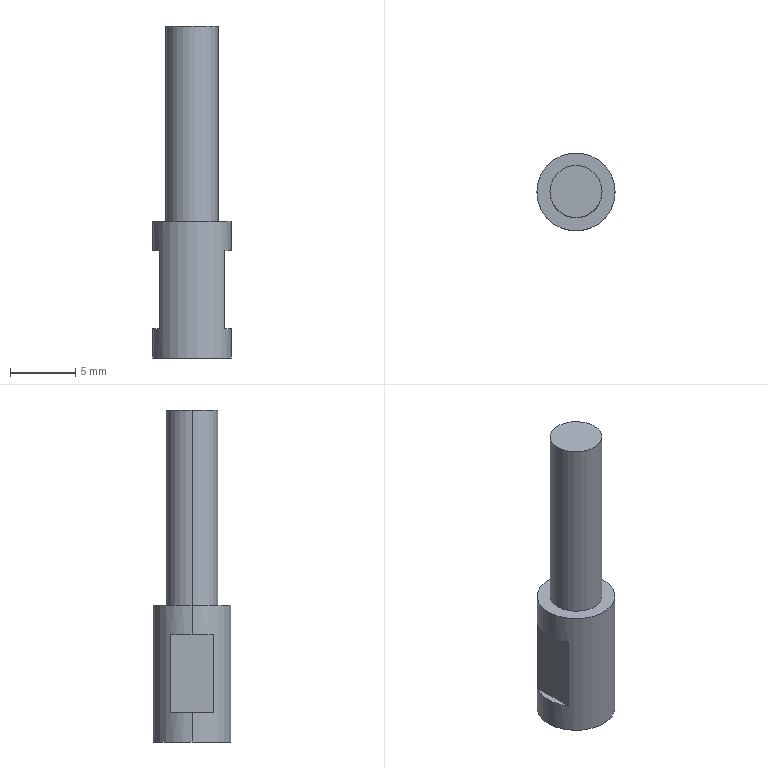Part | STEP file | GLSJ-10-20 | 1 solid | 17 faces | box 6 x 6 x 25.5 mm | volume 383.515 mm3 | plane 9 | cylinder 6 | cone 2 | commonest cylinder face diameters 3.3 x2 4 x2 6 x2
STEP:
#1=CARTESIAN_POINT('',(0.,0.,0.));
#2=DIRECTION('',(0.,0.,1.));
#3=DIRECTION('',(1.,0.,0.));
#4=AXIS2_PLACEMENT_3D('',#1,#2,#3);
#5=CARTESIAN_POINT('',(-1.65,0.,10.));
#6=VERTEX_POINT('',#5);
#7=CARTESIAN_POINT('',(-1.65,0.,0.));
#8=VERTEX_POINT('',#7);
#9=CARTESIAN_POINT('',(-1.65,0.,0.));
#10=DIRECTION('',(0.,0.,-1.));
#11=VECTOR('',#10,1.);
#12=LINE('',#9,#11);
#13=CARTESIAN_POINT('',(0.,0.,0.));
#14=DIRECTION('',(0.,0.,-1.));
#15=DIRECTION('',(-1.,0.,0.));
#16=AXIS2_PLACEMENT_3D('',#13,#14,#15);
#17=CYLINDRICAL_SURFACE('',#16,1.65);
#18=CARTESIAN_POINT('',(6.283,0.));
#19=DIRECTION('',(0.,1.));
#20=VECTOR('',#19,1.);
#21=LINE('',#18,#20);
#22=(GEOMETRIC_REPRESENTATION_CONTEXT(2)PARAMETRIC_REPRESENTATION_CONTEXT()REPRESENTATION_CONTEXT('',''));
#23=DEFINITIONAL_REPRESENTATION('',(#21),#22);
#24=PCURVE('',#17,#23);
#25=CARTESIAN_POINT('',(0.,0.,0.));
#26=DIRECTION('',(0.,0.,-1.));
#27=DIRECTION('',(-1.,0.,0.));
#28=AXIS2_PLACEMENT_3D('',#25,#26,#27);
#29=CYLINDRICAL_SURFACE('',#28,1.65);
#30=CARTESIAN_POINT('',(0.,0.));
#31=DIRECTION('',(0.,1.));
#32=VECTOR('',#31,1.);
#33=LINE('',#30,#32);
#34=(GEOMETRIC_REPRESENTATION_CONTEXT(2)PARAMETRIC_REPRESENTATION_CONTEXT()REPRESENTATION_CONTEXT('',''));
#35=DEFINITIONAL_REPRESENTATION('',(#33),#34);
#36=PCURVE('',#29,#35);
#37=SURFACE_CURVE('',#12,(#24,#36),.PCURVE_S1.);
#38=EDGE_CURVE('',#6,#8,#37,.T.);
#39=ORIENTED_EDGE('',*,*,#38,.T.);
#40=CARTESIAN_POINT('',(1.65,0.,0.));
#41=VERTEX_POINT('',#40);
#42=CARTESIAN_POINT('',(0.,0.,0.));
#43=DIRECTION('',(0.,0.,-1.));
#44=DIRECTION('',(-1.,0.,0.));
#45=AXIS2_PLACEMENT_3D('',#42,#43,#44);
#46=CIRCLE('',#45,1.65);
#47=CARTESIAN_POINT('',(0.,0.));
#48=DIRECTION('',(1.,0.));
#49=VECTOR('',#48,1.);
#50=LINE('',#47,#49);
#51=(GEOMETRIC_REPRESENTATION_CONTEXT(2)PARAMETRIC_REPRESENTATION_CONTEXT()REPRESENTATION_CONTEXT('',''));
#52=DEFINITIONAL_REPRESENTATION('',(#50),#51);
#53=PCURVE('',#17,#52);
#54=CARTESIAN_POINT('',(0.,0.,0.));
#55=DIRECTION('',(0.,0.,1.));
#56=DIRECTION('',(1.,0.,0.));
#57=AXIS2_PLACEMENT_3D('',#54,#55,#56);
#58=PLANE('',#57);
#59=CARTESIAN_POINT('',(-1.65,0.));
#60=CARTESIAN_POINT('',(-1.65,2.858));
#61=CARTESIAN_POINT('',(0.825,1.429));
#62=CARTESIAN_POINT('',(3.3,0.));
#63=CARTESIAN_POINT('',(0.825,-1.429));
#64=CARTESIAN_POINT('',(-1.65,-2.858));
#65=CARTESIAN_POINT('',(-1.65,0.));
#66=(BOUNDED_CURVE()B_SPLINE_CURVE(2,(#59,#60,#61,#62,#63,#64,#65),.UNSPECIFIED.,.T.,.F.)B_SPLINE_CURVE_WITH_KNOTS((1,2,2,2,2,1),(-2.094,0.,2.094,4.189,6.283,8.378),.UNSPECIFIED.)CURVE()GEOMETRIC_REPRESENTATION_ITEM()RATIONAL_B_SPLINE_CURVE((1.,0.5,1.,0.5,1.,0.5,1.))REPRESENTATION_ITEM(''));
#67=(GEOMETRIC_REPRESENTATION_CONTEXT(2)PARAMETRIC_REPRESENTATION_CONTEXT()REPRESENTATION_CONTEXT('',''));
#68=DEFINITIONAL_REPRESENTATION('',(#66),#67);
#69=PCURVE('',#58,#68);
#70=SURFACE_CURVE('',#46,(#53,#69),.PCURVE_S1.);
#71=EDGE_CURVE('',#41,#8,#70,.T.);
#72=ORIENTED_EDGE('',*,*,#71,.F.);
#73=CARTESIAN_POINT('',(1.65,0.,10.));
#74=VERTEX_POINT('',#73);
#75=CARTESIAN_POINT('',(1.65,0.,0.));
#76=DIRECTION('',(0.,0.,-1.));
#77=VECTOR('',#76,1.);
#78=LINE('',#75,#77);
#79=CARTESIAN_POINT('',(3.142,0.));
#80=DIRECTION('',(0.,1.));
#81=VECTOR('',#80,1.);
#82=LINE('',#79,#81);
#83=(GEOMETRIC_REPRESENTATION_CONTEXT(2)PARAMETRIC_REPRESENTATION_CONTEXT()REPRESENTATION_CONTEXT('',''));
#84=DEFINITIONAL_REPRESENTATION('',(#82),#83);
#85=PCURVE('',#17,#84);
#86=CARTESIAN_POINT('',(3.142,0.));
#87=DIRECTION('',(0.,1.));
#88=VECTOR('',#87,1.);
#89=LINE('',#86,#88);
#90=(GEOMETRIC_REPRESENTATION_CONTEXT(2)PARAMETRIC_REPRESENTATION_CONTEXT()REPRESENTATION_CONTEXT('',''));
#91=DEFINITIONAL_REPRESENTATION('',(#89),#90);
#92=PCURVE('',#29,#91);
#93=SURFACE_CURVE('',#78,(#85,#92),.PCURVE_S1.);
#94=EDGE_CURVE('',#74,#41,#93,.T.);
#95=ORIENTED_EDGE('',*,*,#94,.F.);
#96=CARTESIAN_POINT('',(0.,0.,10.));
#97=DIRECTION('',(0.,0.,-1.));
#98=DIRECTION('',(-1.,0.,0.));
#99=AXIS2_PLACEMENT_3D('',#96,#97,#98);
#100=CIRCLE('',#99,1.65);
#101=CARTESIAN_POINT('',(0.,-10.));
#102=DIRECTION('',(1.,0.));
#103=VECTOR('',#102,1.);
#104=LINE('',#101,#103);
#105=(GEOMETRIC_REPRESENTATION_CONTEXT(2)PARAMETRIC_REPRESENTATION_CONTEXT()REPRESENTATION_CONTEXT('',''));
#106=DEFINITIONAL_REPRESENTATION('',(#104),#105);
#107=PCURVE('',#17,#106);
#108=CARTESIAN_POINT('',(0.,0.,10.));
#109=DIRECTION('',(0.,0.,-1.));
#110=DIRECTION('',(-1.,0.,0.));
#111=AXIS2_PLACEMENT_3D('',#108,#109,#110);
#112=CONICAL_SURFACE('',#111,1.65,1.03);
#113=CARTESIAN_POINT('',(0.,0.));
#114=DIRECTION('',(1.,0.));
#115=VECTOR('',#114,1.);
#116=LINE('',#113,#115);
#117=(GEOMETRIC_REPRESENTATION_CONTEXT(2)PARAMETRIC_REPRESENTATION_CONTEXT()REPRESENTATION_CONTEXT('',''));
#118=DEFINITIONAL_REPRESENTATION('',(#116),#117);
#119=PCURVE('',#112,#118);
#120=SURFACE_CURVE('',#100,(#107,#119),.PCURVE_S1.);
#121=EDGE_CURVE('',#74,#6,#120,.T.);
#122=ORIENTED_EDGE('',*,*,#121,.T.);
#123=EDGE_LOOP('',(#39,#72,#95,#122));
#124=FACE_BOUND('',#123,.F.);
#125=ADVANCED_FACE('',(#124),#17,.F.);
#126=ORIENTED_EDGE('',*,*,#121,.F.);
#127=CARTESIAN_POINT('',(0.,0.,10.991));
#128=VERTEX_POINT('',#127);
#129=CARTESIAN_POINT('',(1.65,0.,10.));
#130=DIRECTION('',(0.8572,0.,-0.515));
#131=VECTOR('',#130,1.);
#132=LINE('',#129,#131);
#133=CARTESIAN_POINT('',(3.142,-0.9914));
#134=CARTESIAN_POINT('',(3.142,-0.9764));
#135=CARTESIAN_POINT('',(3.142,-0.9464));
#136=CARTESIAN_POINT('',(3.142,-0.9013));
#137=CARTESIAN_POINT('',(3.142,-0.8562));
#138=CARTESIAN_POINT('',(3.142,-0.8112));
#139=CARTESIAN_POINT('',(3.142,-0.7661));
#140=CARTESIAN_POINT('',(3.142,-0.721));
#141=CARTESIAN_POINT('',(3.142,-0.676));
#142=CARTESIAN_POINT('',(3.142,-0.6309));
#143=CARTESIAN_POINT('',(3.142,-0.5858));
#144=CARTESIAN_POINT('',(3.142,-0.5408));
#145=CARTESIAN_POINT('',(3.142,-0.4957));
#146=CARTESIAN_POINT('',(3.142,-0.4506));
#147=CARTESIAN_POINT('',(3.142,-0.4056));
#148=CARTESIAN_POINT('',(3.142,-0.3605));
#149=CARTESIAN_POINT('',(3.142,-0.3155));
#150=CARTESIAN_POINT('',(3.142,-0.2704));
#151=CARTESIAN_POINT('',(3.142,-0.2253));
#152=CARTESIAN_POINT('',(3.142,-0.1803));
#153=CARTESIAN_POINT('',(3.142,-0.1352));
#154=CARTESIAN_POINT('',(3.142,-0.09013));
#155=CARTESIAN_POINT('',(3.142,-0.04506));
#156=CARTESIAN_POINT('',(3.142,-0.01502));
#157=CARTESIAN_POINT('',(3.142,0.));
#158=B_SPLINE_CURVE_WITH_KNOTS('',3,(#133,#134,#135,#136,#137,#138,#139,#140,#141,#142,#143,#144,#145,#146,#147,#148,#149,#150,#151,#152,#153,#154,#155,#156,#157),.UNSPECIFIED.,.F.,.F.,(4,1,1,1,1,1,1,1,1,1,1,1,1,1,1,1,1,1,1,1,1,1,4),(-1.925,-1.837,-1.75,-1.662,-1.575,-1.487,-1.4,-1.312,-1.225,-1.137,-1.05,-0.9625,-0.875,-0.7875,-0.7,-0.6125,-0.525,-0.4375,-0.35,-0.2625,-0.175,-0.0875,0.),.QUASI_UNIFORM_KNOTS.);
#159=(GEOMETRIC_REPRESENTATION_CONTEXT(2)PARAMETRIC_REPRESENTATION_CONTEXT()REPRESENTATION_CONTEXT('',''));
#160=DEFINITIONAL_REPRESENTATION('',(#158),#159);
#161=PCURVE('',#112,#160);
#162=CARTESIAN_POINT('',(0.,0.,10.));
#163=DIRECTION('',(0.,0.,-1.));
#164=DIRECTION('',(-1.,0.,0.));
#165=AXIS2_PLACEMENT_3D('',#162,#163,#164);
#166=CONICAL_SURFACE('',#165,1.65,1.03);
#167=CARTESIAN_POINT('',(3.142,-0.9914));
#168=CARTESIAN_POINT('',(3.142,-0.9764));
#169=CARTESIAN_POINT('',(3.142,-0.9464));
#170=CARTESIAN_POINT('',(3.142,-0.9013));
#171=CARTESIAN_POINT('',(3.142,-0.8562));
#172=CARTESIAN_POINT('',(3.142,-0.8112));
#173=CARTESIAN_POINT('',(3.142,-0.7661));
#174=CARTESIAN_POINT('',(3.142,-0.721));
#175=CARTESIAN_POINT('',(3.142,-0.676));
#176=CARTESIAN_POINT('',(3.142,-0.6309));
#177=CARTESIAN_POINT('',(3.142,-0.5858));
#178=CARTESIAN_POINT('',(3.142,-0.5408));
#179=CARTESIAN_POINT('',(3.142,-0.4957));
#180=CARTESIAN_POINT('',(3.142,-0.4506));
#181=CARTESIAN_POINT('',(3.142,-0.4056));
#182=CARTESIAN_POINT('',(3.142,-0.3605));
#183=CARTESIAN_POINT('',(3.142,-0.3155));
#184=CARTESIAN_POINT('',(3.142,-0.2704));
#185=CARTESIAN_POINT('',(3.142,-0.2253));
#186=CARTESIAN_POINT('',(3.142,-0.1803));
#187=CARTESIAN_POINT('',(3.142,-0.1352));
#188=CARTESIAN_POINT('',(3.142,-0.09013));
#189=CARTESIAN_POINT('',(3.142,-0.04506));
#190=CARTESIAN_POINT('',(3.142,-0.01502));
#191=CARTESIAN_POINT('',(3.142,0.));
#192=B_SPLINE_CURVE_WITH_KNOTS('',3,(#167,#168,#169,#170,#171,#172,#173,#174,#175,#176,#177,#178,#179,#180,#181,#182,#183,#184,#185,#186,#187,#188,#189,#190,#191),.UNSPECIFIED.,.F.,.F.,(4,1,1,1,1,1,1,1,1,1,1,1,1,1,1,1,1,1,1,1,1,1,4),(-1.925,-1.837,-1.75,-1.662,-1.575,-1.487,-1.4,-1.312,-1.225,-1.137,-1.05,-0.9625,-0.875,-0.7875,-0.7,-0.6125,-0.525,-0.4375,-0.35,-0.2625,-0.175,-0.0875,0.),.QUASI_UNIFORM_KNOTS.);
#193=(GEOMETRIC_REPRESENTATION_CONTEXT(2)PARAMETRIC_REPRESENTATION_CONTEXT()REPRESENTATION_CONTEXT('',''));
#194=DEFINITIONAL_REPRESENTATION('',(#192),#193);
#195=PCURVE('',#166,#194);
#196=SURFACE_CURVE('',#132,(#161,#195),.PCURVE_S1.);
#197=EDGE_CURVE('',#128,#74,#196,.T.);
#198=ORIENTED_EDGE('',*,*,#197,.F.);
#199=CARTESIAN_POINT('',(-1.65,0.,10.));
#200=DIRECTION('',(-0.8572,0.,-0.515));
#201=VECTOR('',#200,1.);
#202=LINE('',#199,#201);
#203=CARTESIAN_POINT('',(6.283,0.));
#204=DIRECTION('',(0.,1.));
#205=VECTOR('',#204,1.);
#206=LINE('',#203,#205);
#207=(GEOMETRIC_REPRESENTATION_CONTEXT(2)PARAMETRIC_REPRESENTATION_CONTEXT()REPRESENTATION_CONTEXT('',''));
#208=DEFINITIONAL_REPRESENTATION('',(#206),#207);
#209=PCURVE('',#112,#208);
#210=CARTESIAN_POINT('',(0.,0.));
#211=DIRECTION('',(0.,1.));
#212=VECTOR('',#211,1.);
#213=LINE('',#210,#212);
#214=(GEOMETRIC_REPRESENTATION_CONTEXT(2)PARAMETRIC_REPRESENTATION_CONTEXT()REPRESENTATION_CONTEXT('',''));
#215=DEFINITIONAL_REPRESENTATION('',(#213),#214);
#216=PCURVE('',#166,#215);
#217=SURFACE_CURVE('',#202,(#209,#216),.PCURVE_S1.);
#218=EDGE_CURVE('',#128,#6,#217,.T.);
#219=ORIENTED_EDGE('',*,*,#218,.T.);
#220=EDGE_LOOP('',(#126,#198,#219));
#221=FACE_BOUND('',#220,.F.);
#222=ADVANCED_FACE('',(#221),#112,.F.);
#223=CARTESIAN_POINT('',(2.,0.,10.5));
#224=VERTEX_POINT('',#223);
#225=CARTESIAN_POINT('',(-2.,0.,10.5));
#226=VERTEX_POINT('',#225);
#227=CARTESIAN_POINT('',(0.,0.,10.5));
#228=DIRECTION('',(0.,0.,1.));
#229=DIRECTION('',(1.,0.,0.));
#230=AXIS2_PLACEMENT_3D('',#227,#228,#229);
#231=CIRCLE('',#230,2.);
#232=CARTESIAN_POINT('',(0.,0.,10.5));
#233=DIRECTION('',(0.,0.,1.));
#234=DIRECTION('',(1.,0.,0.));
#235=AXIS2_PLACEMENT_3D('',#232,#233,#234);
#236=CYLINDRICAL_SURFACE('',#235,2.);
#237=CARTESIAN_POINT('',(0.,0.));
#238=DIRECTION('',(1.,0.));
#239=VECTOR('',#238,1.);
#240=LINE('',#237,#239);
#241=(GEOMETRIC_REPRESENTATION_CONTEXT(2)PARAMETRIC_REPRESENTATION_CONTEXT()REPRESENTATION_CONTEXT('',''));
#242=DEFINITIONAL_REPRESENTATION('',(#240),#241);
#243=PCURVE('',#236,#242);
#244=CARTESIAN_POINT('',(0.,0.,10.5));
#245=DIRECTION('',(0.,0.,1.));
#246=DIRECTION('',(1.,0.,0.));
#247=AXIS2_PLACEMENT_3D('',#244,#245,#246);
#248=PLANE('',#247);
#249=CARTESIAN_POINT('',(0.,0.));
#250=DIRECTION('',(1.,0.));
#251=AXIS2_PLACEMENT_2D('',#249,#250);
#252=CIRCLE('',#251,2.);
#253=(GEOMETRIC_REPRESENTATION_CONTEXT(2)PARAMETRIC_REPRESENTATION_CONTEXT()REPRESENTATION_CONTEXT('',''));
#254=DEFINITIONAL_REPRESENTATION('',(#252),#253);
#255=PCURVE('',#248,#254);
#256=SURFACE_CURVE('',#231,(#243,#255),.PCURVE_S1.);
#257=EDGE_CURVE('',#224,#226,#256,.T.);
#258=ORIENTED_EDGE('',*,*,#257,.T.);
#259=CARTESIAN_POINT('',(-2.,0.,25.5));
#260=VERTEX_POINT('',#259);
#261=CARTESIAN_POINT('',(-2.,0.,10.5));
#262=DIRECTION('',(0.,0.,1.));
#263=VECTOR('',#262,1.);
#264=LINE('',#261,#263);
#265=CARTESIAN_POINT('',(3.142,0.));
#266=DIRECTION('',(0.,1.));
#267=VECTOR('',#266,1.);
#268=LINE('',#265,#267);
#269=(GEOMETRIC_REPRESENTATION_CONTEXT(2)PARAMETRIC_REPRESENTATION_CONTEXT()REPRESENTATION_CONTEXT('',''));
#270=DEFINITIONAL_REPRESENTATION('',(#268),#269);
#271=PCURVE('',#236,#270);
#272=CARTESIAN_POINT('',(0.,0.,10.5));
#273=DIRECTION('',(0.,0.,1.));
#274=DIRECTION('',(1.,0.,0.));
#275=AXIS2_PLACEMENT_3D('',#272,#273,#274);
#276=CYLINDRICAL_SURFACE('',#275,2.);
#277=CARTESIAN_POINT('',(3.142,0.));
#278=DIRECTION('',(0.,1.));
#279=VECTOR('',#278,1.);
#280=LINE('',#277,#279);
#281=(GEOMETRIC_REPRESENTATION_CONTEXT(2)PARAMETRIC_REPRESENTATION_CONTEXT()REPRESENTATION_CONTEXT('',''));
#282=DEFINITIONAL_REPRESENTATION('',(#280),#281);
#283=PCURVE('',#276,#282);
#284=SURFACE_CURVE('',#264,(#271,#283),.PCURVE_S1.);
#285=EDGE_CURVE('',#226,#260,#284,.T.);
#286=ORIENTED_EDGE('',*,*,#285,.T.);
#287=CARTESIAN_POINT('',(2.,0.,25.5));
#288=VERTEX_POINT('',#287);
#289=CARTESIAN_POINT('',(0.,0.,25.5));
#290=DIRECTION('',(0.,0.,1.));
#291=DIRECTION('',(1.,0.,0.));
#292=AXIS2_PLACEMENT_3D('',#289,#290,#291);
#293=CIRCLE('',#292,2.);
#294=CARTESIAN_POINT('',(0.,15.));
#295=DIRECTION('',(1.,0.));
#296=VECTOR('',#295,1.);
#297=LINE('',#294,#296);
#298=(GEOMETRIC_REPRESENTATION_CONTEXT(2)PARAMETRIC_REPRESENTATION_CONTEXT()REPRESENTATION_CONTEXT('',''));
#299=DEFINITIONAL_REPRESENTATION('',(#297),#298);
#300=PCURVE('',#236,#299);
#301=CARTESIAN_POINT('',(0.,0.,25.5));
#302=DIRECTION('',(0.,0.,1.));
#303=DIRECTION('',(1.,0.,0.));
#304=AXIS2_PLACEMENT_3D('',#301,#302,#303);
#305=PLANE('',#304);
#306=CARTESIAN_POINT('',(0.,0.));
#307=DIRECTION('',(1.,0.));
#308=AXIS2_PLACEMENT_2D('',#306,#307);
#309=CIRCLE('',#308,2.);
#310=(GEOMETRIC_REPRESENTATION_CONTEXT(2)PARAMETRIC_REPRESENTATION_CONTEXT()REPRESENTATION_CONTEXT('',''));
#311=DEFINITIONAL_REPRESENTATION('',(#309),#310);
#312=PCURVE('',#305,#311);
#313=SURFACE_CURVE('',#293,(#300,#312),.PCURVE_S1.);
#314=EDGE_CURVE('',#288,#260,#313,.T.);
#315=ORIENTED_EDGE('',*,*,#314,.F.);
#316=CARTESIAN_POINT('',(2.,0.,10.5));
#317=DIRECTION('',(0.,0.,1.));
#318=VECTOR('',#317,1.);
#319=LINE('',#316,#318);
#320=CARTESIAN_POINT('',(0.,0.));
#321=DIRECTION('',(0.,1.));
#322=VECTOR('',#321,1.);
#323=LINE('',#320,#322);
#324=(GEOMETRIC_REPRESENTATION_CONTEXT(2)PARAMETRIC_REPRESENTATION_CONTEXT()REPRESENTATION_CONTEXT('',''));
#325=DEFINITIONAL_REPRESENTATION('',(#323),#324);
#326=PCURVE('',#236,#325);
#327=CARTESIAN_POINT('',(6.283,0.));
#328=DIRECTION('',(0.,1.));
#329=VECTOR('',#328,1.);
#330=LINE('',#327,#329);
#331=(GEOMETRIC_REPRESENTATION_CONTEXT(2)PARAMETRIC_REPRESENTATION_CONTEXT()REPRESENTATION_CONTEXT('',''));
#332=DEFINITIONAL_REPRESENTATION('',(#330),#331);
#333=PCURVE('',#276,#332);
#334=SURFACE_CURVE('',#319,(#326,#333),.PCURVE_S1.);
#335=EDGE_CURVE('',#224,#288,#334,.T.);
#336=ORIENTED_EDGE('',*,*,#335,.F.);
#337=EDGE_LOOP('',(#258,#286,#315,#336));
#338=FACE_BOUND('',#337,.T.);
#339=ADVANCED_FACE('',(#338),#236,.T.);
#340=CARTESIAN_POINT('',(3.,0.,10.5));
#341=VERTEX_POINT('',#340);
#342=CARTESIAN_POINT('',(-3.,0.,10.5));
#343=VERTEX_POINT('',#342);
#344=CARTESIAN_POINT('',(0.,0.,10.5));
#345=DIRECTION('',(0.,0.,1.));
#346=DIRECTION('',(1.,0.,0.));
#347=AXIS2_PLACEMENT_3D('',#344,#345,#346);
#348=CIRCLE('',#347,3.);
#349=CARTESIAN_POINT('',(0.,0.,25.5));
#350=DIRECTION('',(0.,0.,-1.));
#351=DIRECTION('',(-1.,0.,0.));
#352=AXIS2_PLACEMENT_3D('',#349,#350,#351);
#353=CYLINDRICAL_SURFACE('',#352,3.);
#354=CARTESIAN_POINT('',(3.142,15.));
#355=DIRECTION('',(-1.,0.));
#356=VECTOR('',#355,1.);
#357=LINE('',#354,#356);
#358=(GEOMETRIC_REPRESENTATION_CONTEXT(2)PARAMETRIC_REPRESENTATION_CONTEXT()REPRESENTATION_CONTEXT('',''));
#359=DEFINITIONAL_REPRESENTATION('',(#357),#358);
#360=PCURVE('',#353,#359);
#361=CARTESIAN_POINT('',(0.,0.));
#362=DIRECTION('',(1.,0.));
#363=AXIS2_PLACEMENT_2D('',#361,#362);
#364=CIRCLE('',#363,3.);
#365=(GEOMETRIC_REPRESENTATION_CONTEXT(2)PARAMETRIC_REPRESENTATION_CONTEXT()REPRESENTATION_CONTEXT('',''));
#366=DEFINITIONAL_REPRESENTATION('',(#364),#365);
#367=PCURVE('',#248,#366);
#368=SURFACE_CURVE('',#348,(#360,#367),.PCURVE_S1.);
#369=EDGE_CURVE('',#341,#343,#368,.T.);
#370=ORIENTED_EDGE('',*,*,#369,.F.);
#371=CARTESIAN_POINT('',(3.,0.,8.25));
#372=VERTEX_POINT('',#371);
#373=CARTESIAN_POINT('',(3.,0.,25.5));
#374=DIRECTION('',(0.,0.,-1.));
#375=VECTOR('',#374,1.);
#376=LINE('',#373,#375);
#377=CARTESIAN_POINT('',(3.142,0.));
#378=DIRECTION('',(0.,1.));
#379=VECTOR('',#378,1.);
#380=LINE('',#377,#379);
#381=(GEOMETRIC_REPRESENTATION_CONTEXT(2)PARAMETRIC_REPRESENTATION_CONTEXT()REPRESENTATION_CONTEXT('',''));
#382=DEFINITIONAL_REPRESENTATION('',(#380),#381);
#383=PCURVE('',#353,#382);
#384=CARTESIAN_POINT('',(0.,0.,25.5));
#385=DIRECTION('',(0.,0.,-1.));
#386=DIRECTION('',(-1.,0.,0.));
#387=AXIS2_PLACEMENT_3D('',#384,#385,#386);
#388=CYLINDRICAL_SURFACE('',#387,3.);
#389=CARTESIAN_POINT('',(3.142,0.));
#390=DIRECTION('',(0.,1.));
#391=VECTOR('',#390,1.);
#392=LINE('',#389,#391);
#393=(GEOMETRIC_REPRESENTATION_CONTEXT(2)PARAMETRIC_REPRESENTATION_CONTEXT()REPRESENTATION_CONTEXT('',''));
#394=DEFINITIONAL_REPRESENTATION('',(#392),#393);
#395=PCURVE('',#388,#394);
#396=SURFACE_CURVE('',#376,(#383,#395),.PCURVE_S1.);
#397=EDGE_CURVE('',#341,#372,#396,.T.);
#398=ORIENTED_EDGE('',*,*,#397,.T.);
#399=CARTESIAN_POINT('',(2.5,1.658,8.25));
#400=VERTEX_POINT('',#399);
#401=CARTESIAN_POINT('',(0.,0.,8.25));
#402=DIRECTION('',(0.,0.,1.));
#403=DIRECTION('',(1.,0.,0.));
#404=AXIS2_PLACEMENT_3D('',#401,#402,#403);
#405=CIRCLE('',#404,3.);
#406=CARTESIAN_POINT('',(3.142,17.25));
#407=DIRECTION('',(-1.,0.));
#408=VECTOR('',#407,1.);
#409=LINE('',#406,#408);
#410=(GEOMETRIC_REPRESENTATION_CONTEXT(2)PARAMETRIC_REPRESENTATION_CONTEXT()REPRESENTATION_CONTEXT('',''));
#411=DEFINITIONAL_REPRESENTATION('',(#409),#410);
#412=PCURVE('',#353,#411);
#413=CARTESIAN_POINT('',(2.5,-10.,8.25));
#414=DIRECTION('',(0.,0.,1.));
#415=DIRECTION('',(1.,0.,0.));
#416=AXIS2_PLACEMENT_3D('',#413,#414,#415);
#417=PLANE('',#416);
#418=CARTESIAN_POINT('',(-2.5,10.));
#419=DIRECTION('',(1.,0.));
#420=AXIS2_PLACEMENT_2D('',#418,#419);
#421=CIRCLE('',#420,3.);
#422=(GEOMETRIC_REPRESENTATION_CONTEXT(2)PARAMETRIC_REPRESENTATION_CONTEXT()REPRESENTATION_CONTEXT('',''));
#423=DEFINITIONAL_REPRESENTATION('',(#421),#422);
#424=PCURVE('',#417,#423);
#425=SURFACE_CURVE('',#405,(#412,#424),.PCURVE_S1.);
#426=EDGE_CURVE('',#372,#400,#425,.T.);
#427=ORIENTED_EDGE('',*,*,#426,.T.);
#428=CARTESIAN_POINT('',(2.5,1.658,2.25));
#429=VERTEX_POINT('',#428);
#430=CARTESIAN_POINT('',(2.5,1.658,25.5));
#431=DIRECTION('',(0.,0.,-1.));
#432=VECTOR('',#431,1.);
#433=LINE('',#430,#432);
#434=CARTESIAN_POINT('',(2.556,0.));
#435=DIRECTION('',(0.,1.));
#436=VECTOR('',#435,1.);
#437=LINE('',#434,#436);
#438=(GEOMETRIC_REPRESENTATION_CONTEXT(2)PARAMETRIC_REPRESENTATION_CONTEXT()REPRESENTATION_CONTEXT('',''));
#439=DEFINITIONAL_REPRESENTATION('',(#437),#438);
#440=PCURVE('',#353,#439);
#441=CARTESIAN_POINT('',(2.5,-10.,2.25));
#442=DIRECTION('',(-1.,0.,0.));
#443=DIRECTION('',(0.,0.,1.));
#444=AXIS2_PLACEMENT_3D('',#441,#442,#443);
#445=PLANE('',#444);
#446=CARTESIAN_POINT('',(23.25,11.658));
#447=DIRECTION('',(-1.,0.));
#448=VECTOR('',#447,1.);
#449=LINE('',#446,#448);
#450=(GEOMETRIC_REPRESENTATION_CONTEXT(2)PARAMETRIC_REPRESENTATION_CONTEXT()REPRESENTATION_CONTEXT('',''));
#451=DEFINITIONAL_REPRESENTATION('',(#449),#450);
#452=PCURVE('',#445,#451);
#453=SURFACE_CURVE('',#433,(#440,#452),.PCURVE_S1.);
#454=EDGE_CURVE('',#400,#429,#453,.T.);
#455=ORIENTED_EDGE('',*,*,#454,.T.);
#456=CARTESIAN_POINT('',(3.,0.,2.25));
#457=VERTEX_POINT('',#456);
#458=CARTESIAN_POINT('',(0.,0.,2.25));
#459=DIRECTION('',(0.,0.,-1.));
#460=DIRECTION('',(-1.,0.,0.));
#461=AXIS2_PLACEMENT_3D('',#458,#459,#460);
#462=CIRCLE('',#461,3.);
#463=CARTESIAN_POINT('',(0.,23.25));
#464=DIRECTION('',(1.,0.));
#465=VECTOR('',#464,1.);
#466=LINE('',#463,#465);
#467=(GEOMETRIC_REPRESENTATION_CONTEXT(2)PARAMETRIC_REPRESENTATION_CONTEXT()REPRESENTATION_CONTEXT('',''));
#468=DEFINITIONAL_REPRESENTATION('',(#466),#467);
#469=PCURVE('',#353,#468);
#470=CARTESIAN_POINT('',(2.5,-10.,2.25));
#471=DIRECTION('',(0.,0.,-1.));
#472=DIRECTION('',(-1.,0.,0.));
#473=AXIS2_PLACEMENT_3D('',#470,#471,#472);
#474=PLANE('',#473);
#475=CARTESIAN_POINT('',(2.5,10.));
#476=DIRECTION('',(1.,0.));
#477=AXIS2_PLACEMENT_2D('',#475,#476);
#478=CIRCLE('',#477,3.);
#479=(GEOMETRIC_REPRESENTATION_CONTEXT(2)PARAMETRIC_REPRESENTATION_CONTEXT()REPRESENTATION_CONTEXT('',''));
#480=DEFINITIONAL_REPRESENTATION('',(#478),#479);
#481=PCURVE('',#474,#480);
#482=SURFACE_CURVE('',#462,(#469,#481),.PCURVE_S1.);
#483=EDGE_CURVE('',#429,#457,#482,.T.);
#484=ORIENTED_EDGE('',*,*,#483,.T.);
#485=CARTESIAN_POINT('',(3.,0.,0.));
#486=VERTEX_POINT('',#485);
#487=CARTESIAN_POINT('',(3.,0.,25.5));
#488=DIRECTION('',(0.,0.,-1.));
#489=VECTOR('',#488,1.);
#490=LINE('',#487,#489);
#491=CARTESIAN_POINT('',(3.142,0.));
#492=DIRECTION('',(0.,1.));
#493=VECTOR('',#492,1.);
#494=LINE('',#491,#493);
#495=(GEOMETRIC_REPRESENTATION_CONTEXT(2)PARAMETRIC_REPRESENTATION_CONTEXT()REPRESENTATION_CONTEXT('',''));
#496=DEFINITIONAL_REPRESENTATION('',(#494),#495);
#497=PCURVE('',#353,#496);
#498=CARTESIAN_POINT('',(3.142,0.));
#499=DIRECTION('',(0.,1.));
#500=VECTOR('',#499,1.);
#501=LINE('',#498,#500);
#502=(GEOMETRIC_REPRESENTATION_CONTEXT(2)PARAMETRIC_REPRESENTATION_CONTEXT()REPRESENTATION_CONTEXT('',''));
#503=DEFINITIONAL_REPRESENTATION('',(#501),#502);
#504=PCURVE('',#388,#503);
#505=SURFACE_CURVE('',#490,(#497,#504),.PCURVE_S1.);
#506=EDGE_CURVE('',#457,#486,#505,.T.);
#507=ORIENTED_EDGE('',*,*,#506,.T.);
#508=CARTESIAN_POINT('',(-3.,0.,0.));
#509=VERTEX_POINT('',#508);
#510=CARTESIAN_POINT('',(0.,0.,0.));
#511=DIRECTION('',(0.,0.,1.));
#512=DIRECTION('',(1.,0.,0.));
#513=AXIS2_PLACEMENT_3D('',#510,#511,#512);
#514=CIRCLE('',#513,3.);
#515=CARTESIAN_POINT('',(3.142,25.5));
#516=DIRECTION('',(-1.,0.));
#517=VECTOR('',#516,1.);
#518=LINE('',#515,#517);
#519=(GEOMETRIC_REPRESENTATION_CONTEXT(2)PARAMETRIC_REPRESENTATION_CONTEXT()REPRESENTATION_CONTEXT('',''));
#520=DEFINITIONAL_REPRESENTATION('',(#518),#519);
#521=PCURVE('',#353,#520);
#522=CARTESIAN_POINT('',(0.,0.));
#523=DIRECTION('',(1.,0.));
#524=AXIS2_PLACEMENT_2D('',#522,#523);
#525=CIRCLE('',#524,3.);
#526=(GEOMETRIC_REPRESENTATION_CONTEXT(2)PARAMETRIC_REPRESENTATION_CONTEXT()REPRESENTATION_CONTEXT('',''));
#527=DEFINITIONAL_REPRESENTATION('',(#525),#526);
#528=PCURVE('',#58,#527);
#529=SURFACE_CURVE('',#514,(#521,#528),.PCURVE_S1.);
#530=EDGE_CURVE('',#486,#509,#529,.T.);
#531=ORIENTED_EDGE('',*,*,#530,.T.);
#532=CARTESIAN_POINT('',(-3.,0.,2.25));
#533=VERTEX_POINT('',#532);
#534=CARTESIAN_POINT('',(-3.,0.,25.5));
#535=DIRECTION('',(0.,0.,-1.));
#536=VECTOR('',#535,1.);
#537=LINE('',#534,#536);
#538=CARTESIAN_POINT('',(0.,0.));
#539=DIRECTION('',(0.,1.));
#540=VECTOR('',#539,1.);
#541=LINE('',#538,#540);
#542=(GEOMETRIC_REPRESENTATION_CONTEXT(2)PARAMETRIC_REPRESENTATION_CONTEXT()REPRESENTATION_CONTEXT('',''));
#543=DEFINITIONAL_REPRESENTATION('',(#541),#542);
#544=PCURVE('',#353,#543);
#545=CARTESIAN_POINT('',(6.283,0.));
#546=DIRECTION('',(0.,1.));
#547=VECTOR('',#546,1.);
#548=LINE('',#545,#547);
#549=(GEOMETRIC_REPRESENTATION_CONTEXT(2)PARAMETRIC_REPRESENTATION_CONTEXT()REPRESENTATION_CONTEXT('',''));
#550=DEFINITIONAL_REPRESENTATION('',(#548),#549);
#551=PCURVE('',#388,#550);
#552=SURFACE_CURVE('',#537,(#544,#551),.PCURVE_S1.);
#553=EDGE_CURVE('',#533,#509,#552,.T.);
#554=ORIENTED_EDGE('',*,*,#553,.F.);
#555=CARTESIAN_POINT('',(-2.5,1.658,2.25));
#556=VERTEX_POINT('',#555);
#557=CARTESIAN_POINT('',(0.,0.,2.25));
#558=DIRECTION('',(0.,0.,-1.));
#559=DIRECTION('',(-1.,0.,0.));
#560=AXIS2_PLACEMENT_3D('',#557,#558,#559);
#561=CIRCLE('',#560,3.);
#562=CARTESIAN_POINT('',(0.,23.25));
#563=DIRECTION('',(1.,0.));
#564=VECTOR('',#563,1.);
#565=LINE('',#562,#564);
#566=(GEOMETRIC_REPRESENTATION_CONTEXT(2)PARAMETRIC_REPRESENTATION_CONTEXT()REPRESENTATION_CONTEXT('',''));
#567=DEFINITIONAL_REPRESENTATION('',(#565),#566);
#568=PCURVE('',#353,#567);
#569=CARTESIAN_POINT('',(-2.5,-10.,2.25));
#570=DIRECTION('',(0.,0.,-1.));
#571=DIRECTION('',(-1.,0.,0.));
#572=AXIS2_PLACEMENT_3D('',#569,#570,#571);
#573=PLANE('',#572);
#574=CARTESIAN_POINT('',(-2.5,10.));
#575=DIRECTION('',(1.,0.));
#576=AXIS2_PLACEMENT_2D('',#574,#575);
#577=CIRCLE('',#576,3.);
#578=(GEOMETRIC_REPRESENTATION_CONTEXT(2)PARAMETRIC_REPRESENTATION_CONTEXT()REPRESENTATION_CONTEXT('',''));
#579=DEFINITIONAL_REPRESENTATION('',(#577),#578);
#580=PCURVE('',#573,#579);
#581=SURFACE_CURVE('',#561,(#568,#580),.PCURVE_S1.);
#582=EDGE_CURVE('',#533,#556,#581,.T.);
#583=ORIENTED_EDGE('',*,*,#582,.T.);
#584=CARTESIAN_POINT('',(-2.5,1.658,8.25));
#585=VERTEX_POINT('',#584);
#586=CARTESIAN_POINT('',(-2.5,1.658,25.5));
#587=DIRECTION('',(0.,0.,1.));
#588=VECTOR('',#587,1.);
#589=LINE('',#586,#588);
#590=CARTESIAN_POINT('',(0.5857,0.));
#591=DIRECTION('',(0.,-1.));
#592=VECTOR('',#591,1.);
#593=LINE('',#590,#592);
#594=(GEOMETRIC_REPRESENTATION_CONTEXT(2)PARAMETRIC_REPRESENTATION_CONTEXT()REPRESENTATION_CONTEXT('',''));
#595=DEFINITIONAL_REPRESENTATION('',(#593),#594);
#596=PCURVE('',#353,#595);
#597=CARTESIAN_POINT('',(-2.5,-10.,2.25));
#598=DIRECTION('',(1.,0.,0.));
#599=DIRECTION('',(0.,0.,-1.));
#600=AXIS2_PLACEMENT_3D('',#597,#598,#599);
#601=PLANE('',#600);
#602=CARTESIAN_POINT('',(-23.25,11.658));
#603=DIRECTION('',(-1.,0.));
#604=VECTOR('',#603,1.);
#605=LINE('',#602,#604);
#606=(GEOMETRIC_REPRESENTATION_CONTEXT(2)PARAMETRIC_REPRESENTATION_CONTEXT()REPRESENTATION_CONTEXT('',''));
#607=DEFINITIONAL_REPRESENTATION('',(#605),#606);
#608=PCURVE('',#601,#607);
#609=SURFACE_CURVE('',#589,(#596,#608),.PCURVE_S1.);
#610=EDGE_CURVE('',#556,#585,#609,.T.);
#611=ORIENTED_EDGE('',*,*,#610,.T.);
#612=CARTESIAN_POINT('',(-3.,0.,8.25));
#613=VERTEX_POINT('',#612);
#614=CARTESIAN_POINT('',(0.,0.,8.25));
#615=DIRECTION('',(0.,0.,1.));
#616=DIRECTION('',(1.,0.,0.));
#617=AXIS2_PLACEMENT_3D('',#614,#615,#616);
#618=CIRCLE('',#617,3.);
#619=CARTESIAN_POINT('',(3.142,17.25));
#620=DIRECTION('',(-1.,0.));
#621=VECTOR('',#620,1.);
#622=LINE('',#619,#621);
#623=(GEOMETRIC_REPRESENTATION_CONTEXT(2)PARAMETRIC_REPRESENTATION_CONTEXT()REPRESENTATION_CONTEXT('',''));
#624=DEFINITIONAL_REPRESENTATION('',(#622),#623);
#625=PCURVE('',#353,#624);
#626=CARTESIAN_POINT('',(-2.5,-10.,8.25));
#627=DIRECTION('',(0.,0.,1.));
#628=DIRECTION('',(1.,0.,0.));
#629=AXIS2_PLACEMENT_3D('',#626,#627,#628);
#630=PLANE('',#629);
#631=CARTESIAN_POINT('',(2.5,10.));
#632=DIRECTION('',(1.,0.));
#633=AXIS2_PLACEMENT_2D('',#631,#632);
#634=CIRCLE('',#633,3.);
#635=(GEOMETRIC_REPRESENTATION_CONTEXT(2)PARAMETRIC_REPRESENTATION_CONTEXT()REPRESENTATION_CONTEXT('',''));
#636=DEFINITIONAL_REPRESENTATION('',(#634),#635);
#637=PCURVE('',#630,#636);
#638=SURFACE_CURVE('',#618,(#625,#637),.PCURVE_S1.);
#639=EDGE_CURVE('',#585,#613,#638,.T.);
#640=ORIENTED_EDGE('',*,*,#639,.T.);
#641=CARTESIAN_POINT('',(-3.,0.,25.5));
#642=DIRECTION('',(0.,0.,-1.));
#643=VECTOR('',#642,1.);
#644=LINE('',#641,#643);
#645=CARTESIAN_POINT('',(0.,0.));
#646=DIRECTION('',(0.,1.));
#647=VECTOR('',#646,1.);
#648=LINE('',#645,#647);
#649=(GEOMETRIC_REPRESENTATION_CONTEXT(2)PARAMETRIC_REPRESENTATION_CONTEXT()REPRESENTATION_CONTEXT('',''));
#650=DEFINITIONAL_REPRESENTATION('',(#648),#649);
#651=PCURVE('',#353,#650);
#652=CARTESIAN_POINT('',(6.283,0.));
#653=DIRECTION('',(0.,1.));
#654=VECTOR('',#653,1.);
#655=LINE('',#652,#654);
#656=(GEOMETRIC_REPRESENTATION_CONTEXT(2)PARAMETRIC_REPRESENTATION_CONTEXT()REPRESENTATION_CONTEXT('',''));
#657=DEFINITIONAL_REPRESENTATION('',(#655),#656);
#658=PCURVE('',#388,#657);
#659=SURFACE_CURVE('',#644,(#651,#658),.PCURVE_S1.);
#660=EDGE_CURVE('',#343,#613,#659,.T.);
#661=ORIENTED_EDGE('',*,*,#660,.F.);
#662=EDGE_LOOP('',(#370,#398,#427,#455,#484,#507,#531,#554,#583,#611,#640,#661));
#663=FACE_BOUND('',#662,.T.);
#664=ADVANCED_FACE('',(#663),#353,.T.);
#665=ORIENTED_EDGE('',*,*,#397,.F.);
#666=CARTESIAN_POINT('',(0.,0.,10.5));
#667=DIRECTION('',(0.,0.,1.));
#668=DIRECTION('',(1.,0.,0.));
#669=AXIS2_PLACEMENT_3D('',#666,#667,#668);
#670=CIRCLE('',#669,3.);
#671=CARTESIAN_POINT('',(9.425,15.));
#672=DIRECTION('',(-1.,0.));
#673=VECTOR('',#672,1.);
#674=LINE('',#671,#673);
#675=(GEOMETRIC_REPRESENTATION_CONTEXT(2)PARAMETRIC_REPRESENTATION_CONTEXT()REPRESENTATION_CONTEXT('',''));
#676=DEFINITIONAL_REPRESENTATION('',(#674),#675);
#677=PCURVE('',#388,#676);
#678=CARTESIAN_POINT('',(0.,0.));
#679=DIRECTION('',(1.,0.));
#680=AXIS2_PLACEMENT_2D('',#678,#679);
#681=CIRCLE('',#680,3.);
#682=(GEOMETRIC_REPRESENTATION_CONTEXT(2)PARAMETRIC_REPRESENTATION_CONTEXT()REPRESENTATION_CONTEXT('',''));
#683=DEFINITIONAL_REPRESENTATION('',(#681),#682);
#684=PCURVE('',#248,#683);
#685=SURFACE_CURVE('',#670,(#677,#684),.PCURVE_S1.);
#686=EDGE_CURVE('',#343,#341,#685,.T.);
#687=ORIENTED_EDGE('',*,*,#686,.F.);
#688=ORIENTED_EDGE('',*,*,#660,.T.);
#689=CARTESIAN_POINT('',(-2.5,-1.658,8.25));
#690=VERTEX_POINT('',#689);
#691=CARTESIAN_POINT('',(0.,0.,8.25));
#692=DIRECTION('',(0.,0.,1.));
#693=DIRECTION('',(1.,0.,0.));
#694=AXIS2_PLACEMENT_3D('',#691,#692,#693);
#695=CIRCLE('',#694,3.);
#696=CARTESIAN_POINT('',(9.425,17.25));
#697=DIRECTION('',(-1.,0.));
#698=VECTOR('',#697,1.);
#699=LINE('',#696,#698);
#700=(GEOMETRIC_REPRESENTATION_CONTEXT(2)PARAMETRIC_REPRESENTATION_CONTEXT()REPRESENTATION_CONTEXT('',''));
#701=DEFINITIONAL_REPRESENTATION('',(#699),#700);
#702=PCURVE('',#388,#701);
#703=CARTESIAN_POINT('',(2.5,10.));
#704=DIRECTION('',(1.,0.));
#705=AXIS2_PLACEMENT_2D('',#703,#704);
#706=CIRCLE('',#705,3.);
#707=(GEOMETRIC_REPRESENTATION_CONTEXT(2)PARAMETRIC_REPRESENTATION_CONTEXT()REPRESENTATION_CONTEXT('',''));
#708=DEFINITIONAL_REPRESENTATION('',(#706),#707);
#709=PCURVE('',#630,#708);
#710=SURFACE_CURVE('',#695,(#702,#709),.PCURVE_S1.);
#711=EDGE_CURVE('',#613,#690,#710,.T.);
#712=ORIENTED_EDGE('',*,*,#711,.T.);
#713=CARTESIAN_POINT('',(-2.5,-1.658,2.25));
#714=VERTEX_POINT('',#713);
#715=CARTESIAN_POINT('',(-2.5,-1.658,25.5));
#716=DIRECTION('',(0.,0.,-1.));
#717=VECTOR('',#716,1.);
#718=LINE('',#715,#717);
#719=CARTESIAN_POINT('',(5.697,0.));
#720=DIRECTION('',(0.,1.));
#721=VECTOR('',#720,1.);
#722=LINE('',#719,#721);
#723=(GEOMETRIC_REPRESENTATION_CONTEXT(2)PARAMETRIC_REPRESENTATION_CONTEXT()REPRESENTATION_CONTEXT('',''));
#724=DEFINITIONAL_REPRESENTATION('',(#722),#723);
#725=PCURVE('',#388,#724);
#726=CARTESIAN_POINT('',(-23.25,8.342));
#727=DIRECTION('',(1.,0.));
#728=VECTOR('',#727,1.);
#729=LINE('',#726,#728);
#730=(GEOMETRIC_REPRESENTATION_CONTEXT(2)PARAMETRIC_REPRESENTATION_CONTEXT()REPRESENTATION_CONTEXT('',''));
#731=DEFINITIONAL_REPRESENTATION('',(#729),#730);
#732=PCURVE('',#601,#731);
#733=SURFACE_CURVE('',#718,(#725,#732),.PCURVE_S1.);
#734=EDGE_CURVE('',#690,#714,#733,.T.);
#735=ORIENTED_EDGE('',*,*,#734,.T.);
#736=CARTESIAN_POINT('',(0.,0.,2.25));
#737=DIRECTION('',(0.,0.,-1.));
#738=DIRECTION('',(-1.,0.,0.));
#739=AXIS2_PLACEMENT_3D('',#736,#737,#738);
#740=CIRCLE('',#739,3.);
#741=CARTESIAN_POINT('',(0.,23.25));
#742=DIRECTION('',(1.,0.));
#743=VECTOR('',#742,1.);
#744=LINE('',#741,#743);
#745=(GEOMETRIC_REPRESENTATION_CONTEXT(2)PARAMETRIC_REPRESENTATION_CONTEXT()REPRESENTATION_CONTEXT('',''));
#746=DEFINITIONAL_REPRESENTATION('',(#744),#745);
#747=PCURVE('',#388,#746);
#748=CARTESIAN_POINT('',(-2.5,10.));
#749=DIRECTION('',(1.,0.));
#750=AXIS2_PLACEMENT_2D('',#748,#749);
#751=CIRCLE('',#750,3.);
#752=(GEOMETRIC_REPRESENTATION_CONTEXT(2)PARAMETRIC_REPRESENTATION_CONTEXT()REPRESENTATION_CONTEXT('',''));
#753=DEFINITIONAL_REPRESENTATION('',(#751),#752);
#754=PCURVE('',#573,#753);
#755=SURFACE_CURVE('',#740,(#747,#754),.PCURVE_S1.);
#756=EDGE_CURVE('',#714,#533,#755,.T.);
#757=ORIENTED_EDGE('',*,*,#756,.T.);
#758=ORIENTED_EDGE('',*,*,#553,.T.);
#759=CARTESIAN_POINT('',(0.,0.,0.));
#760=DIRECTION('',(0.,0.,1.));
#761=DIRECTION('',(1.,0.,0.));
#762=AXIS2_PLACEMENT_3D('',#759,#760,#761);
#763=CIRCLE('',#762,3.);
#764=CARTESIAN_POINT('',(9.425,25.5));
#765=DIRECTION('',(-1.,0.));
#766=VECTOR('',#765,1.);
#767=LINE('',#764,#766);
#768=(GEOMETRIC_REPRESENTATION_CONTEXT(2)PARAMETRIC_REPRESENTATION_CONTEXT()REPRESENTATION_CONTEXT('',''));
#769=DEFINITIONAL_REPRESENTATION('',(#767),#768);
#770=PCURVE('',#388,#769);
#771=CARTESIAN_POINT('',(0.,0.));
#772=DIRECTION('',(1.,0.));
#773=AXIS2_PLACEMENT_2D('',#771,#772);
#774=CIRCLE('',#773,3.);
#775=(GEOMETRIC_REPRESENTATION_CONTEXT(2)PARAMETRIC_REPRESENTATION_CONTEXT()REPRESENTATION_CONTEXT('',''));
#776=DEFINITIONAL_REPRESENTATION('',(#774),#775);
#777=PCURVE('',#58,#776);
#778=SURFACE_CURVE('',#763,(#770,#777),.PCURVE_S1.);
#779=EDGE_CURVE('',#509,#486,#778,.T.);
#780=ORIENTED_EDGE('',*,*,#779,.T.);
#781=ORIENTED_EDGE('',*,*,#506,.F.);
#782=CARTESIAN_POINT('',(2.5,-1.658,2.25));
#783=VERTEX_POINT('',#782);
#784=CARTESIAN_POINT('',(0.,0.,2.25));
#785=DIRECTION('',(0.,0.,-1.));
#786=DIRECTION('',(-1.,0.,0.));
#787=AXIS2_PLACEMENT_3D('',#784,#785,#786);
#788=CIRCLE('',#787,3.);
#789=CARTESIAN_POINT('',(0.,23.25));
#790=DIRECTION('',(1.,0.));
#791=VECTOR('',#790,1.);
#792=LINE('',#789,#791);
#793=(GEOMETRIC_REPRESENTATION_CONTEXT(2)PARAMETRIC_REPRESENTATION_CONTEXT()REPRESENTATION_CONTEXT('',''));
#794=DEFINITIONAL_REPRESENTATION('',(#792),#793);
#795=PCURVE('',#388,#794);
#796=CARTESIAN_POINT('',(2.5,10.));
#797=DIRECTION('',(1.,0.));
#798=AXIS2_PLACEMENT_2D('',#796,#797);
#799=CIRCLE('',#798,3.);
#800=(GEOMETRIC_REPRESENTATION_CONTEXT(2)PARAMETRIC_REPRESENTATION_CONTEXT()REPRESENTATION_CONTEXT('',''));
#801=DEFINITIONAL_REPRESENTATION('',(#799),#800);
#802=PCURVE('',#474,#801);
#803=SURFACE_CURVE('',#788,(#795,#802),.PCURVE_S1.);
#804=EDGE_CURVE('',#457,#783,#803,.T.);
#805=ORIENTED_EDGE('',*,*,#804,.T.);
#806=CARTESIAN_POINT('',(2.5,-1.658,8.25));
#807=VERTEX_POINT('',#806);
#808=CARTESIAN_POINT('',(2.5,-1.658,25.5));
#809=DIRECTION('',(0.,0.,1.));
#810=VECTOR('',#809,1.);
#811=LINE('',#808,#810);
#812=CARTESIAN_POINT('',(3.727,0.));
#813=DIRECTION('',(0.,-1.));
#814=VECTOR('',#813,1.);
#815=LINE('',#812,#814);
#816=(GEOMETRIC_REPRESENTATION_CONTEXT(2)PARAMETRIC_REPRESENTATION_CONTEXT()REPRESENTATION_CONTEXT('',''));
#817=DEFINITIONAL_REPRESENTATION('',(#815),#816);
#818=PCURVE('',#388,#817);
#819=CARTESIAN_POINT('',(23.25,8.342));
#820=DIRECTION('',(1.,0.));
#821=VECTOR('',#820,1.);
#822=LINE('',#819,#821);
#823=(GEOMETRIC_REPRESENTATION_CONTEXT(2)PARAMETRIC_REPRESENTATION_CONTEXT()REPRESENTATION_CONTEXT('',''));
#824=DEFINITIONAL_REPRESENTATION('',(#822),#823);
#825=PCURVE('',#445,#824);
#826=SURFACE_CURVE('',#811,(#818,#825),.PCURVE_S1.);
#827=EDGE_CURVE('',#783,#807,#826,.T.);
#828=ORIENTED_EDGE('',*,*,#827,.T.);
#829=CARTESIAN_POINT('',(0.,0.,8.25));
#830=DIRECTION('',(0.,0.,1.));
#831=DIRECTION('',(1.,0.,0.));
#832=AXIS2_PLACEMENT_3D('',#829,#830,#831);
#833=CIRCLE('',#832,3.);
#834=CARTESIAN_POINT('',(9.425,17.25));
#835=DIRECTION('',(-1.,0.));
#836=VECTOR('',#835,1.);
#837=LINE('',#834,#836);
#838=(GEOMETRIC_REPRESENTATION_CONTEXT(2)PARAMETRIC_REPRESENTATION_CONTEXT()REPRESENTATION_CONTEXT('',''));
#839=DEFINITIONAL_REPRESENTATION('',(#837),#838);
#840=PCURVE('',#388,#839);
#841=CARTESIAN_POINT('',(-2.5,10.));
#842=DIRECTION('',(1.,0.));
#843=AXIS2_PLACEMENT_2D('',#841,#842);
#844=CIRCLE('',#843,3.);
#845=(GEOMETRIC_REPRESENTATION_CONTEXT(2)PARAMETRIC_REPRESENTATION_CONTEXT()REPRESENTATION_CONTEXT('',''));
#846=DEFINITIONAL_REPRESENTATION('',(#844),#845);
#847=PCURVE('',#417,#846);
#848=SURFACE_CURVE('',#833,(#840,#847),.PCURVE_S1.);
#849=EDGE_CURVE('',#807,#372,#848,.T.);
#850=ORIENTED_EDGE('',*,*,#849,.T.);
#851=EDGE_LOOP('',(#665,#687,#688,#712,#735,#757,#758,#780,#781,#805,#828,#850));
#852=FACE_BOUND('',#851,.T.);
#853=ADVANCED_FACE('',(#852),#388,.T.);
#854=CARTESIAN_POINT('',(0.,0.,0.));
#855=DIRECTION('',(0.,0.,-1.));
#856=DIRECTION('',(-1.,0.,0.));
#857=AXIS2_PLACEMENT_3D('',#854,#855,#856);
#858=CIRCLE('',#857,1.65);
#859=CARTESIAN_POINT('',(-1.65,0.));
#860=CARTESIAN_POINT('',(-1.65,2.858));
#861=CARTESIAN_POINT('',(0.825,1.429));
#862=CARTESIAN_POINT('',(3.3,0.));
#863=CARTESIAN_POINT('',(0.825,-1.429));
#864=CARTESIAN_POINT('',(-1.65,-2.858));
#865=CARTESIAN_POINT('',(-1.65,0.));
#866=(BOUNDED_CURVE()B_SPLINE_CURVE(2,(#859,#860,#861,#862,#863,#864,#865),.UNSPECIFIED.,.T.,.F.)B_SPLINE_CURVE_WITH_KNOTS((1,2,2,2,2,1),(-2.094,0.,2.094,4.189,6.283,8.378),.UNSPECIFIED.)CURVE()GEOMETRIC_REPRESENTATION_ITEM()RATIONAL_B_SPLINE_CURVE((1.,0.5,1.,0.5,1.,0.5,1.))REPRESENTATION_ITEM(''));
#867=(GEOMETRIC_REPRESENTATION_CONTEXT(2)PARAMETRIC_REPRESENTATION_CONTEXT()REPRESENTATION_CONTEXT('',''));
#868=DEFINITIONAL_REPRESENTATION('',(#866),#867);
#869=PCURVE('',#58,#868);
#870=CARTESIAN_POINT('',(0.,0.));
#871=DIRECTION('',(1.,0.));
#872=VECTOR('',#871,1.);
#873=LINE('',#870,#872);
#874=(GEOMETRIC_REPRESENTATION_CONTEXT(2)PARAMETRIC_REPRESENTATION_CONTEXT()REPRESENTATION_CONTEXT('',''));
#875=DEFINITIONAL_REPRESENTATION('',(#873),#874);
#876=PCURVE('',#29,#875);
#877=SURFACE_CURVE('',#858,(#869,#876),.PCURVE_S1.);
#878=EDGE_CURVE('',#8,#41,#877,.T.);
#879=ORIENTED_EDGE('',*,*,#878,.F.);
#880=ORIENTED_EDGE('',*,*,#71,.F.);
#881=EDGE_LOOP('',(#879,#880));
#882=FACE_BOUND('',#881,.T.);
#883=ORIENTED_EDGE('',*,*,#779,.F.);
#884=ORIENTED_EDGE('',*,*,#530,.F.);
#885=EDGE_LOOP('',(#883,#884));
#886=FACE_BOUND('',#885,.T.);
#887=ADVANCED_FACE('',(#882,#886),#58,.F.);
#888=ORIENTED_EDGE('',*,*,#257,.F.);
#889=CARTESIAN_POINT('',(0.,0.,10.5));
#890=DIRECTION('',(0.,0.,1.));
#891=DIRECTION('',(1.,0.,0.));
#892=AXIS2_PLACEMENT_3D('',#889,#890,#891);
#893=CIRCLE('',#892,2.);
#894=CARTESIAN_POINT('',(0.,0.));
#895=DIRECTION('',(1.,0.));
#896=AXIS2_PLACEMENT_2D('',#894,#895);
#897=CIRCLE('',#896,2.);
#898=(GEOMETRIC_REPRESENTATION_CONTEXT(2)PARAMETRIC_REPRESENTATION_CONTEXT()REPRESENTATION_CONTEXT('',''));
#899=DEFINITIONAL_REPRESENTATION('',(#897),#898);
#900=PCURVE('',#248,#899);
#901=CARTESIAN_POINT('',(0.,0.));
#902=DIRECTION('',(1.,0.));
#903=VECTOR('',#902,1.);
#904=LINE('',#901,#903);
#905=(GEOMETRIC_REPRESENTATION_CONTEXT(2)PARAMETRIC_REPRESENTATION_CONTEXT()REPRESENTATION_CONTEXT('',''));
#906=DEFINITIONAL_REPRESENTATION('',(#904),#905);
#907=PCURVE('',#276,#906);
#908=SURFACE_CURVE('',#893,(#900,#907),.PCURVE_S1.);
#909=EDGE_CURVE('',#226,#224,#908,.T.);
#910=ORIENTED_EDGE('',*,*,#909,.F.);
#911=EDGE_LOOP('',(#888,#910));
#912=FACE_BOUND('',#911,.T.);
#913=ORIENTED_EDGE('',*,*,#686,.T.);
#914=ORIENTED_EDGE('',*,*,#369,.T.);
#915=EDGE_LOOP('',(#913,#914));
#916=FACE_BOUND('',#915,.T.);
#917=ADVANCED_FACE('',(#912,#916),#248,.T.);
#918=ORIENTED_EDGE('',*,*,#285,.F.);
#919=ORIENTED_EDGE('',*,*,#909,.T.);
#920=ORIENTED_EDGE('',*,*,#335,.T.);
#921=CARTESIAN_POINT('',(0.,0.,25.5));
#922=DIRECTION('',(0.,0.,1.));
#923=DIRECTION('',(1.,0.,0.));
#924=AXIS2_PLACEMENT_3D('',#921,#922,#923);
#925=CIRCLE('',#924,2.);
#926=CARTESIAN_POINT('',(0.,15.));
#927=DIRECTION('',(1.,0.));
#928=VECTOR('',#927,1.);
#929=LINE('',#926,#928);
#930=(GEOMETRIC_REPRESENTATION_CONTEXT(2)PARAMETRIC_REPRESENTATION_CONTEXT()REPRESENTATION_CONTEXT('',''));
#931=DEFINITIONAL_REPRESENTATION('',(#929),#930);
#932=PCURVE('',#276,#931);
#933=CARTESIAN_POINT('',(0.,0.));
#934=DIRECTION('',(1.,0.));
#935=AXIS2_PLACEMENT_2D('',#933,#934);
#936=CIRCLE('',#935,2.);
#937=(GEOMETRIC_REPRESENTATION_CONTEXT(2)PARAMETRIC_REPRESENTATION_CONTEXT()REPRESENTATION_CONTEXT('',''));
#938=DEFINITIONAL_REPRESENTATION('',(#936),#937);
#939=PCURVE('',#305,#938);
#940=SURFACE_CURVE('',#925,(#932,#939),.PCURVE_S1.);
#941=EDGE_CURVE('',#260,#288,#940,.T.);
#942=ORIENTED_EDGE('',*,*,#941,.F.);
#943=EDGE_LOOP('',(#918,#919,#920,#942));
#944=FACE_BOUND('',#943,.T.);
#945=ADVANCED_FACE('',(#944),#276,.T.);
#946=ORIENTED_EDGE('',*,*,#314,.T.);
#947=ORIENTED_EDGE('',*,*,#941,.T.);
#948=EDGE_LOOP('',(#946,#947));
#949=FACE_BOUND('',#948,.T.);
#950=ADVANCED_FACE('',(#949),#305,.T.);
#951=CARTESIAN_POINT('',(0.,0.,10.));
#952=DIRECTION('',(0.,0.,-1.));
#953=DIRECTION('',(-1.,0.,0.));
#954=AXIS2_PLACEMENT_3D('',#951,#952,#953);
#955=CIRCLE('',#954,1.65);
#956=CARTESIAN_POINT('',(0.,0.));
#957=DIRECTION('',(1.,0.));
#958=VECTOR('',#957,1.);
#959=LINE('',#956,#958);
#960=(GEOMETRIC_REPRESENTATION_CONTEXT(2)PARAMETRIC_REPRESENTATION_CONTEXT()REPRESENTATION_CONTEXT('',''));
#961=DEFINITIONAL_REPRESENTATION('',(#959),#960);
#962=PCURVE('',#166,#961);
#963=CARTESIAN_POINT('',(0.,-10.));
#964=DIRECTION('',(1.,0.));
#965=VECTOR('',#964,1.);
#966=LINE('',#963,#965);
#967=(GEOMETRIC_REPRESENTATION_CONTEXT(2)PARAMETRIC_REPRESENTATION_CONTEXT()REPRESENTATION_CONTEXT('',''));
#968=DEFINITIONAL_REPRESENTATION('',(#966),#967);
#969=PCURVE('',#29,#968);
#970=SURFACE_CURVE('',#955,(#962,#969),.PCURVE_S1.);
#971=EDGE_CURVE('',#6,#74,#970,.T.);
#972=ORIENTED_EDGE('',*,*,#971,.F.);
#973=ORIENTED_EDGE('',*,*,#218,.F.);
#974=ORIENTED_EDGE('',*,*,#197,.T.);
#975=EDGE_LOOP('',(#972,#973,#974));
#976=FACE_BOUND('',#975,.F.);
#977=ADVANCED_FACE('',(#976),#166,.F.);
#978=ORIENTED_EDGE('',*,*,#878,.F.);
#979=ORIENTED_EDGE('',*,*,#38,.F.);
#980=ORIENTED_EDGE('',*,*,#971,.T.);
#981=ORIENTED_EDGE('',*,*,#94,.T.);
#982=EDGE_LOOP('',(#978,#979,#980,#981));
#983=FACE_BOUND('',#982,.F.);
#984=ADVANCED_FACE('',(#983),#29,.F.);
#985=CARTESIAN_POINT('',(2.5,-10.,8.25));
#986=DIRECTION('',(0.,1.,0.));
#987=VECTOR('',#986,1.);
#988=LINE('',#985,#987);
#989=CARTESIAN_POINT('',(6.,0.));
#990=DIRECTION('',(0.,1.));
#991=VECTOR('',#990,1.);
#992=LINE('',#989,#991);
#993=(GEOMETRIC_REPRESENTATION_CONTEXT(2)PARAMETRIC_REPRESENTATION_CONTEXT()REPRESENTATION_CONTEXT('',''));
#994=DEFINITIONAL_REPRESENTATION('',(#992),#993);
#995=PCURVE('',#445,#994);
#996=CARTESIAN_POINT('',(0.,0.));
#997=DIRECTION('',(0.,1.));
#998=VECTOR('',#997,1.);
#999=LINE('',#996,#998);
#1000=(GEOMETRIC_REPRESENTATION_CONTEXT(2)PARAMETRIC_REPRESENTATION_CONTEXT()REPRESENTATION_CONTEXT('',''));
#1001=DEFINITIONAL_REPRESENTATION('',(#999),#1000);
#1002=PCURVE('',#417,#1001);
#1003=SURFACE_CURVE('',#988,(#995,#1002),.PCURVE_S1.);
#1004=EDGE_CURVE('',#807,#400,#1003,.T.);
#1005=ORIENTED_EDGE('',*,*,#1004,.F.);
#1006=ORIENTED_EDGE('',*,*,#827,.F.);
#1007=CARTESIAN_POINT('',(2.5,-10.,2.25));
#1008=DIRECTION('',(0.,1.,0.));
#1009=VECTOR('',#1008,1.);
#1010=LINE('',#1007,#1009);
#1011=CARTESIAN_POINT('',(0.,0.));
#1012=DIRECTION('',(0.,1.));
#1013=VECTOR('',#1012,1.);
#1014=LINE('',#1011,#1013);
#1015=(GEOMETRIC_REPRESENTATION_CONTEXT(2)PARAMETRIC_REPRESENTATION_CONTEXT()REPRESENTATION_CONTEXT('',''));
#1016=DEFINITIONAL_REPRESENTATION('',(#1014),#1015);
#1017=PCURVE('',#445,#1016);
#1018=CARTESIAN_POINT('',(0.,0.));
#1019=DIRECTION('',(0.,1.));
#1020=VECTOR('',#1019,1.);
#1021=LINE('',#1018,#1020);
#1022=(GEOMETRIC_REPRESENTATION_CONTEXT(2)PARAMETRIC_REPRESENTATION_CONTEXT()REPRESENTATION_CONTEXT('',''));
#1023=DEFINITIONAL_REPRESENTATION('',(#1021),#1022);
#1024=PCURVE('',#474,#1023);
#1025=SURFACE_CURVE('',#1010,(#1017,#1024),.PCURVE_S1.);
#1026=EDGE_CURVE('',#783,#429,#1025,.T.);
#1027=ORIENTED_EDGE('',*,*,#1026,.T.);
#1028=ORIENTED_EDGE('',*,*,#454,.F.);
#1029=EDGE_LOOP('',(#1005,#1006,#1027,#1028));
#1030=FACE_BOUND('',#1029,.T.);
#1031=ADVANCED_FACE('',(#1030),#445,.F.);
#1032=ORIENTED_EDGE('',*,*,#1026,.F.);
#1033=ORIENTED_EDGE('',*,*,#804,.F.);
#1034=ORIENTED_EDGE('',*,*,#483,.F.);
#1035=EDGE_LOOP('',(#1032,#1033,#1034));
#1036=FACE_BOUND('',#1035,.T.);
#1037=ADVANCED_FACE('',(#1036),#474,.F.);
#1038=ORIENTED_EDGE('',*,*,#1004,.T.);
#1039=ORIENTED_EDGE('',*,*,#426,.F.);
#1040=ORIENTED_EDGE('',*,*,#849,.F.);
#1041=EDGE_LOOP('',(#1038,#1039,#1040));
#1042=FACE_BOUND('',#1041,.T.);
#1043=ADVANCED_FACE('',(#1042),#417,.F.);
#1044=CARTESIAN_POINT('',(-2.5,-10.,2.25));
#1045=DIRECTION('',(0.,1.,0.));
#1046=VECTOR('',#1045,1.);
#1047=LINE('',#1044,#1046);
#1048=CARTESIAN_POINT('',(0.,0.));
#1049=DIRECTION('',(0.,1.));
#1050=VECTOR('',#1049,1.);
#1051=LINE('',#1048,#1050);
#1052=(GEOMETRIC_REPRESENTATION_CONTEXT(2)PARAMETRIC_REPRESENTATION_CONTEXT()REPRESENTATION_CONTEXT('',''));
#1053=DEFINITIONAL_REPRESENTATION('',(#1051),#1052);
#1054=PCURVE('',#573,#1053);
#1055=CARTESIAN_POINT('',(0.,0.));
#1056=DIRECTION('',(0.,1.));
#1057=VECTOR('',#1056,1.);
#1058=LINE('',#1055,#1057);
#1059=(GEOMETRIC_REPRESENTATION_CONTEXT(2)PARAMETRIC_REPRESENTATION_CONTEXT()REPRESENTATION_CONTEXT('',''));
#1060=DEFINITIONAL_REPRESENTATION('',(#1058),#1059);
#1061=PCURVE('',#601,#1060);
#1062=SURFACE_CURVE('',#1047,(#1054,#1061),.PCURVE_S1.);
#1063=EDGE_CURVE('',#714,#556,#1062,.T.);
#1064=ORIENTED_EDGE('',*,*,#1063,.T.);
#1065=ORIENTED_EDGE('',*,*,#582,.F.);
#1066=ORIENTED_EDGE('',*,*,#756,.F.);
#1067=EDGE_LOOP('',(#1064,#1065,#1066));
#1068=FACE_BOUND('',#1067,.T.);
#1069=ADVANCED_FACE('',(#1068),#573,.F.);
#1070=CARTESIAN_POINT('',(-2.5,-10.,8.25));
#1071=DIRECTION('',(0.,1.,0.));
#1072=VECTOR('',#1071,1.);
#1073=LINE('',#1070,#1072);
#1074=CARTESIAN_POINT('',(-6.,0.));
#1075=DIRECTION('',(0.,1.));
#1076=VECTOR('',#1075,1.);
#1077=LINE('',#1074,#1076);
#1078=(GEOMETRIC_REPRESENTATION_CONTEXT(2)PARAMETRIC_REPRESENTATION_CONTEXT()REPRESENTATION_CONTEXT('',''));
#1079=DEFINITIONAL_REPRESENTATION('',(#1077),#1078);
#1080=PCURVE('',#601,#1079);
#1081=CARTESIAN_POINT('',(0.,0.));
#1082=DIRECTION('',(0.,1.));
#1083=VECTOR('',#1082,1.);
#1084=LINE('',#1081,#1083);
#1085=(GEOMETRIC_REPRESENTATION_CONTEXT(2)PARAMETRIC_REPRESENTATION_CONTEXT()REPRESENTATION_CONTEXT('',''));
#1086=DEFINITIONAL_REPRESENTATION('',(#1084),#1085);
#1087=PCURVE('',#630,#1086);
#1088=SURFACE_CURVE('',#1073,(#1080,#1087),.PCURVE_S1.);
#1089=EDGE_CURVE('',#690,#585,#1088,.T.);
#1090=ORIENTED_EDGE('',*,*,#1089,.T.);
#1091=ORIENTED_EDGE('',*,*,#610,.F.);
#1092=ORIENTED_EDGE('',*,*,#1063,.F.);
#1093=ORIENTED_EDGE('',*,*,#734,.F.);
#1094=EDGE_LOOP('',(#1090,#1091,#1092,#1093));
#1095=FACE_BOUND('',#1094,.T.);
#1096=ADVANCED_FACE('',(#1095),#601,.F.);
#1097=ORIENTED_EDGE('',*,*,#1089,.F.);
#1098=ORIENTED_EDGE('',*,*,#711,.F.);
#1099=ORIENTED_EDGE('',*,*,#639,.F.);
#1100=EDGE_LOOP('',(#1097,#1098,#1099));
#1101=FACE_BOUND('',#1100,.T.);
#1102=ADVANCED_FACE('',(#1101),#630,.F.);
#1103=CLOSED_SHELL('',(#125,#222,#339,#664,#853,#887,#917,#945,#950,#977,#984,#1031,#1037,#1043,#1069,#1096,#1102));
#1104=MANIFOLD_SOLID_BREP('',#1103);
#1105=(LENGTH_UNIT()NAMED_UNIT(*)SI_UNIT(.MILLI.,.METRE.));
#1106=UNCERTAINTY_MEASURE_WITH_UNIT(LENGTH_MEASURE(0.0000001),#1105,'','');
#1107=(NAMED_UNIT(*)PLANE_ANGLE_UNIT()SI_UNIT($,.RADIAN.));
#1108=(NAMED_UNIT(*)SI_UNIT($,.STERADIAN.)SOLID_ANGLE_UNIT());
#1109=(GEOMETRIC_REPRESENTATION_CONTEXT(3)GLOBAL_UNCERTAINTY_ASSIGNED_CONTEXT((#1106))GLOBAL_UNIT_ASSIGNED_CONTEXT((#1105,#1107,#1108))REPRESENTATION_CONTEXT('',''));
#1110=ADVANCED_BREP_SHAPE_REPRESENTATION('',(#4,#1104),#1109);